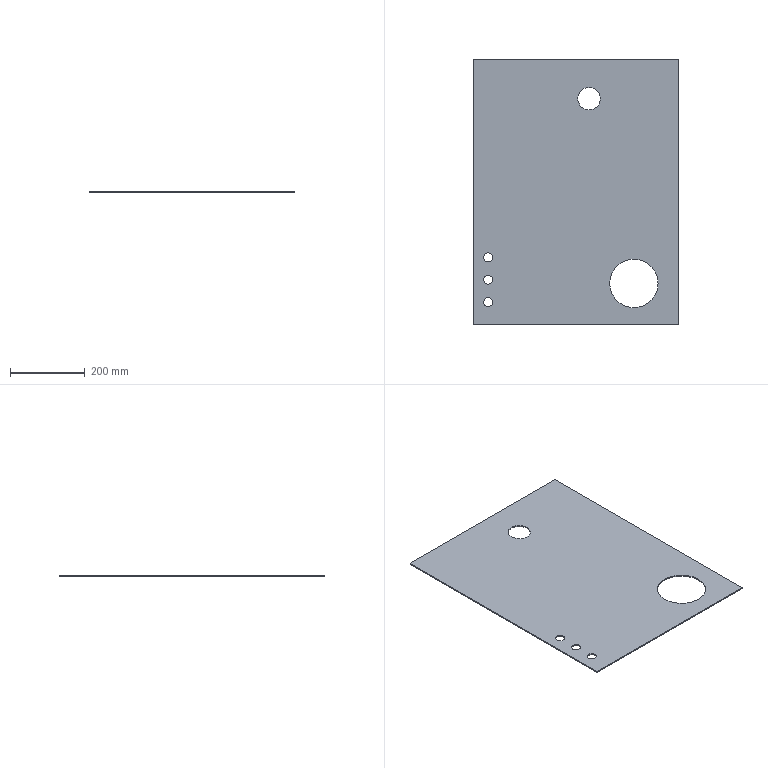Part | SolidWorks | features Extrusion 1 | 1 solid | 20 faces | box 550 x 710 x 3 mm | volume 1118991 mm3 | cylinder 14 | plane 6 | commonest cylinder face diameters 24.2 x6 4 x4 60.2 x2 130 x2
STEP:
#1=CARTESIAN_POINT('',(27.9,180.,3.));
#2=VERTEX_POINT('',#1);
#3=CARTESIAN_POINT('',(52.1,180.,3.));
#4=VERTEX_POINT('',#3);
#5=CARTESIAN_POINT('',(40.,180.,3.));
#6=DIRECTION('',(0.,0.,1.));
#7=DIRECTION('',(1.,0.,0.));
#8=AXIS2_PLACEMENT_3D('',#5,#6,#7);
#9=CIRCLE('',#8,12.1);
#10=EDGE_CURVE('',#2,#4,#9,.T.);
#11=ORIENTED_EDGE('',*,*,#10,.T.);
#12=CARTESIAN_POINT('',(52.1,180.,0.));
#13=VERTEX_POINT('',#12);
#14=CARTESIAN_POINT('',(52.1,180.,3.));
#15=DIRECTION('',(0.,0.,-1.));
#16=VECTOR('',#15,1000.);
#17=LINE('',#14,#16);
#18=EDGE_CURVE('',#4,#13,#17,.T.);
#19=ORIENTED_EDGE('',*,*,#18,.T.);
#20=CARTESIAN_POINT('',(27.9,180.,0.));
#21=VERTEX_POINT('',#20);
#22=CARTESIAN_POINT('',(40.,180.,0.));
#23=DIRECTION('',(0.,0.,1.));
#24=DIRECTION('',(1.,0.,0.));
#25=AXIS2_PLACEMENT_3D('',#22,#23,#24);
#26=CIRCLE('',#25,12.1);
#27=EDGE_CURVE('',#21,#13,#26,.T.);
#28=ORIENTED_EDGE('',*,*,#27,.F.);
#29=CARTESIAN_POINT('',(27.9,180.,3.));
#30=DIRECTION('',(0.,0.,-1.));
#31=VECTOR('',#30,1000.);
#32=LINE('',#29,#31);
#33=EDGE_CURVE('',#2,#21,#32,.T.);
#34=ORIENTED_EDGE('',*,*,#33,.F.);
#35=EDGE_LOOP('',(#11,#19,#28,#34));
#36=FACE_OUTER_BOUND('',#35,.T.);
#37=CARTESIAN_POINT('',(40.,180.,3.));
#38=DIRECTION('',(0.,0.,-1.));
#39=DIRECTION('',(-1.,0.,0.));
#40=AXIS2_PLACEMENT_3D('',#37,#38,#39);
#41=CYLINDRICAL_SURFACE('',#40,12.1);
#42=ADVANCED_FACE('',(#36),#41,.F.);
#43=CARTESIAN_POINT('',(27.9,120.,3.));
#44=VERTEX_POINT('',#43);
#45=CARTESIAN_POINT('',(52.1,120.,3.));
#46=VERTEX_POINT('',#45);
#47=CARTESIAN_POINT('',(40.,120.,3.));
#48=DIRECTION('',(0.,0.,1.));
#49=DIRECTION('',(1.,0.,0.));
#50=AXIS2_PLACEMENT_3D('',#47,#48,#49);
#51=CIRCLE('',#50,12.1);
#52=EDGE_CURVE('',#44,#46,#51,.T.);
#53=ORIENTED_EDGE('',*,*,#52,.T.);
#54=CARTESIAN_POINT('',(52.1,120.,0.));
#55=VERTEX_POINT('',#54);
#56=CARTESIAN_POINT('',(52.1,120.,3.));
#57=DIRECTION('',(0.,0.,-1.));
#58=VECTOR('',#57,1000.);
#59=LINE('',#56,#58);
#60=EDGE_CURVE('',#46,#55,#59,.T.);
#61=ORIENTED_EDGE('',*,*,#60,.T.);
#62=CARTESIAN_POINT('',(27.9,120.,0.));
#63=VERTEX_POINT('',#62);
#64=CARTESIAN_POINT('',(40.,120.,0.));
#65=DIRECTION('',(0.,0.,1.));
#66=DIRECTION('',(1.,0.,0.));
#67=AXIS2_PLACEMENT_3D('',#64,#65,#66);
#68=CIRCLE('',#67,12.1);
#69=EDGE_CURVE('',#63,#55,#68,.T.);
#70=ORIENTED_EDGE('',*,*,#69,.F.);
#71=CARTESIAN_POINT('',(27.9,120.,3.));
#72=DIRECTION('',(0.,0.,-1.));
#73=VECTOR('',#72,1000.);
#74=LINE('',#71,#73);
#75=EDGE_CURVE('',#44,#63,#74,.T.);
#76=ORIENTED_EDGE('',*,*,#75,.F.);
#77=EDGE_LOOP('',(#53,#61,#70,#76));
#78=FACE_OUTER_BOUND('',#77,.T.);
#79=CARTESIAN_POINT('',(40.,120.,3.));
#80=DIRECTION('',(0.,0.,-1.));
#81=DIRECTION('',(-1.,0.,0.));
#82=AXIS2_PLACEMENT_3D('',#79,#80,#81);
#83=CYLINDRICAL_SURFACE('',#82,12.1);
#84=ADVANCED_FACE('',(#78),#83,.F.);
#85=CARTESIAN_POINT('',(279.9,605.,3.));
#86=VERTEX_POINT('',#85);
#87=CARTESIAN_POINT('',(340.1,605.,3.));
#88=VERTEX_POINT('',#87);
#89=CARTESIAN_POINT('',(310.,605.,3.));
#90=DIRECTION('',(0.,0.,1.));
#91=DIRECTION('',(1.,0.,0.));
#92=AXIS2_PLACEMENT_3D('',#89,#90,#91);
#93=CIRCLE('',#92,30.1);
#94=EDGE_CURVE('',#86,#88,#93,.T.);
#95=ORIENTED_EDGE('',*,*,#94,.T.);
#96=CARTESIAN_POINT('',(340.1,605.,0.));
#97=VERTEX_POINT('',#96);
#98=CARTESIAN_POINT('',(340.1,605.,3.));
#99=DIRECTION('',(0.,0.,-1.));
#100=VECTOR('',#99,1000.);
#101=LINE('',#98,#100);
#102=EDGE_CURVE('',#88,#97,#101,.T.);
#103=ORIENTED_EDGE('',*,*,#102,.T.);
#104=CARTESIAN_POINT('',(279.9,605.,0.));
#105=VERTEX_POINT('',#104);
#106=CARTESIAN_POINT('',(310.,605.,0.));
#107=DIRECTION('',(0.,0.,1.));
#108=DIRECTION('',(1.,0.,0.));
#109=AXIS2_PLACEMENT_3D('',#106,#107,#108);
#110=CIRCLE('',#109,30.1);
#111=EDGE_CURVE('',#105,#97,#110,.T.);
#112=ORIENTED_EDGE('',*,*,#111,.F.);
#113=CARTESIAN_POINT('',(279.9,605.,3.));
#114=DIRECTION('',(0.,0.,-1.));
#115=VECTOR('',#114,1000.);
#116=LINE('',#113,#115);
#117=EDGE_CURVE('',#86,#105,#116,.T.);
#118=ORIENTED_EDGE('',*,*,#117,.F.);
#119=EDGE_LOOP('',(#95,#103,#112,#118));
#120=FACE_OUTER_BOUND('',#119,.T.);
#121=CARTESIAN_POINT('',(310.,605.,3.));
#122=DIRECTION('',(0.,0.,-1.));
#123=DIRECTION('',(-1.,0.,0.));
#124=AXIS2_PLACEMENT_3D('',#121,#122,#123);
#125=CYLINDRICAL_SURFACE('',#124,30.1);
#126=ADVANCED_FACE('',(#120),#125,.F.);
#127=CARTESIAN_POINT('',(365.,110.,3.));
#128=VERTEX_POINT('',#127);
#129=CARTESIAN_POINT('',(495.,110.,3.));
#130=VERTEX_POINT('',#129);
#131=CARTESIAN_POINT('',(430.,110.,3.));
#132=DIRECTION('',(0.,0.,1.));
#133=DIRECTION('',(1.,0.,0.));
#134=AXIS2_PLACEMENT_3D('',#131,#132,#133);
#135=CIRCLE('',#134,65.);
#136=EDGE_CURVE('',#128,#130,#135,.T.);
#137=ORIENTED_EDGE('',*,*,#136,.T.);
#138=CARTESIAN_POINT('',(495.,110.,0.));
#139=VERTEX_POINT('',#138);
#140=CARTESIAN_POINT('',(495.,110.,3.));
#141=DIRECTION('',(0.,0.,-1.));
#142=VECTOR('',#141,1000.);
#143=LINE('',#140,#142);
#144=EDGE_CURVE('',#130,#139,#143,.T.);
#145=ORIENTED_EDGE('',*,*,#144,.T.);
#146=CARTESIAN_POINT('',(365.,110.,0.));
#147=VERTEX_POINT('',#146);
#148=CARTESIAN_POINT('',(430.,110.,0.));
#149=DIRECTION('',(0.,0.,1.));
#150=DIRECTION('',(1.,0.,0.));
#151=AXIS2_PLACEMENT_3D('',#148,#149,#150);
#152=CIRCLE('',#151,65.);
#153=EDGE_CURVE('',#147,#139,#152,.T.);
#154=ORIENTED_EDGE('',*,*,#153,.F.);
#155=CARTESIAN_POINT('',(365.,110.,3.));
#156=DIRECTION('',(0.,0.,-1.));
#157=VECTOR('',#156,1000.);
#158=LINE('',#155,#157);
#159=EDGE_CURVE('',#128,#147,#158,.T.);
#160=ORIENTED_EDGE('',*,*,#159,.F.);
#161=EDGE_LOOP('',(#137,#145,#154,#160));
#162=FACE_OUTER_BOUND('',#161,.T.);
#163=CARTESIAN_POINT('',(430.,110.,3.));
#164=DIRECTION('',(0.,0.,-1.));
#165=DIRECTION('',(-1.,0.,0.));
#166=AXIS2_PLACEMENT_3D('',#163,#164,#165);
#167=CYLINDRICAL_SURFACE('',#166,65.);
#168=ADVANCED_FACE('',(#162),#167,.F.);
#169=CARTESIAN_POINT('',(27.9,60.,3.));
#170=VERTEX_POINT('',#169);
#171=CARTESIAN_POINT('',(52.1,60.,3.));
#172=VERTEX_POINT('',#171);
#173=CARTESIAN_POINT('',(40.,60.,3.));
#174=DIRECTION('',(0.,0.,1.));
#175=DIRECTION('',(1.,0.,0.));
#176=AXIS2_PLACEMENT_3D('',#173,#174,#175);
#177=CIRCLE('',#176,12.1);
#178=EDGE_CURVE('',#170,#172,#177,.T.);
#179=ORIENTED_EDGE('',*,*,#178,.T.);
#180=CARTESIAN_POINT('',(52.1,60.,0.));
#181=VERTEX_POINT('',#180);
#182=CARTESIAN_POINT('',(52.1,60.,3.));
#183=DIRECTION('',(0.,0.,-1.));
#184=VECTOR('',#183,1000.);
#185=LINE('',#182,#184);
#186=EDGE_CURVE('',#172,#181,#185,.T.);
#187=ORIENTED_EDGE('',*,*,#186,.T.);
#188=CARTESIAN_POINT('',(27.9,60.,0.));
#189=VERTEX_POINT('',#188);
#190=CARTESIAN_POINT('',(40.,60.,0.));
#191=DIRECTION('',(0.,0.,1.));
#192=DIRECTION('',(1.,0.,0.));
#193=AXIS2_PLACEMENT_3D('',#190,#191,#192);
#194=CIRCLE('',#193,12.1);
#195=EDGE_CURVE('',#189,#181,#194,.T.);
#196=ORIENTED_EDGE('',*,*,#195,.F.);
#197=CARTESIAN_POINT('',(27.9,60.,3.));
#198=DIRECTION('',(0.,0.,-1.));
#199=VECTOR('',#198,1000.);
#200=LINE('',#197,#199);
#201=EDGE_CURVE('',#170,#189,#200,.T.);
#202=ORIENTED_EDGE('',*,*,#201,.F.);
#203=EDGE_LOOP('',(#179,#187,#196,#202));
#204=FACE_OUTER_BOUND('',#203,.T.);
#205=CARTESIAN_POINT('',(40.,60.,3.));
#206=DIRECTION('',(0.,0.,-1.));
#207=DIRECTION('',(-1.,0.,0.));
#208=AXIS2_PLACEMENT_3D('',#205,#206,#207);
#209=CYLINDRICAL_SURFACE('',#208,12.1);
#210=ADVANCED_FACE('',(#204),#209,.F.);
#211=CARTESIAN_POINT('',(2.,710.,3.));
#212=VERTEX_POINT('',#211);
#213=CARTESIAN_POINT('',(0.,708.,3.));
#214=VERTEX_POINT('',#213);
#215=CARTESIAN_POINT('',(2.,708.,3.));
#216=DIRECTION('',(0.,0.,1.));
#217=DIRECTION('',(-1.,0.,0.));
#218=AXIS2_PLACEMENT_3D('',#215,#216,#217);
#219=CIRCLE('',#218,2.);
#220=EDGE_CURVE('',#212,#214,#219,.T.);
#221=ORIENTED_EDGE('',*,*,#220,.T.);
#222=CARTESIAN_POINT('',(0.,2.,3.));
#223=VERTEX_POINT('',#222);
#224=CARTESIAN_POINT('',(0.,2.,3.));
#225=DIRECTION('',(0.,-1.,0.));
#226=VECTOR('',#225,1000.);
#227=LINE('',#224,#226);
#228=EDGE_CURVE('',#214,#223,#227,.T.);
#229=ORIENTED_EDGE('',*,*,#228,.T.);
#230=CARTESIAN_POINT('',(2.,0.,3.));
#231=VERTEX_POINT('',#230);
#232=CARTESIAN_POINT('',(2.,2.,3.));
#233=DIRECTION('',(0.,0.,1.));
#234=DIRECTION('',(-1.,0.,0.));
#235=AXIS2_PLACEMENT_3D('',#232,#233,#234);
#236=CIRCLE('',#235,2.);
#237=EDGE_CURVE('',#223,#231,#236,.T.);
#238=ORIENTED_EDGE('',*,*,#237,.T.);
#239=CARTESIAN_POINT('',(548.,0.,3.));
#240=VERTEX_POINT('',#239);
#241=CARTESIAN_POINT('',(2.,0.,3.));
#242=DIRECTION('',(1.,0.,0.));
#243=VECTOR('',#242,1000.);
#244=LINE('',#241,#243);
#245=EDGE_CURVE('',#231,#240,#244,.T.);
#246=ORIENTED_EDGE('',*,*,#245,.T.);
#247=CARTESIAN_POINT('',(550.,2.,3.));
#248=VERTEX_POINT('',#247);
#249=CARTESIAN_POINT('',(548.,2.,3.));
#250=DIRECTION('',(0.,0.,1.));
#251=DIRECTION('',(1.,0.,0.));
#252=AXIS2_PLACEMENT_3D('',#249,#250,#251);
#253=CIRCLE('',#252,2.);
#254=EDGE_CURVE('',#240,#248,#253,.T.);
#255=ORIENTED_EDGE('',*,*,#254,.T.);
#256=CARTESIAN_POINT('',(550.,708.,3.));
#257=VERTEX_POINT('',#256);
#258=CARTESIAN_POINT('',(550.,2.,3.));
#259=DIRECTION('',(0.,1.,0.));
#260=VECTOR('',#259,1000.);
#261=LINE('',#258,#260);
#262=EDGE_CURVE('',#248,#257,#261,.T.);
#263=ORIENTED_EDGE('',*,*,#262,.T.);
#264=CARTESIAN_POINT('',(548.,710.,3.));
#265=VERTEX_POINT('',#264);
#266=CARTESIAN_POINT('',(548.,708.,3.));
#267=DIRECTION('',(0.,0.,1.));
#268=DIRECTION('',(-1.,0.,0.));
#269=AXIS2_PLACEMENT_3D('',#266,#267,#268);
#270=CIRCLE('',#269,2.);
#271=EDGE_CURVE('',#257,#265,#270,.T.);
#272=ORIENTED_EDGE('',*,*,#271,.T.);
#273=CARTESIAN_POINT('',(2.,710.,3.));
#274=DIRECTION('',(-1.,0.,0.));
#275=VECTOR('',#274,1000.);
#276=LINE('',#273,#275);
#277=EDGE_CURVE('',#265,#212,#276,.T.);
#278=ORIENTED_EDGE('',*,*,#277,.T.);
#279=EDGE_LOOP('',(#221,#229,#238,#246,#255,#263,#272,#278));
#280=FACE_OUTER_BOUND('',#279,.T.);
#281=ORIENTED_EDGE('',*,*,#178,.F.);
#282=CARTESIAN_POINT('',(40.,60.,3.));
#283=DIRECTION('',(0.,0.,1.));
#284=DIRECTION('',(1.,0.,0.));
#285=AXIS2_PLACEMENT_3D('',#282,#283,#284);
#286=CIRCLE('',#285,12.1);
#287=EDGE_CURVE('',#172,#170,#286,.T.);
#288=ORIENTED_EDGE('',*,*,#287,.F.);
#289=EDGE_LOOP('',(#281,#288));
#290=FACE_BOUND('',#289,.T.);
#291=ORIENTED_EDGE('',*,*,#136,.F.);
#292=CARTESIAN_POINT('',(430.,110.,3.));
#293=DIRECTION('',(0.,0.,1.));
#294=DIRECTION('',(1.,0.,0.));
#295=AXIS2_PLACEMENT_3D('',#292,#293,#294);
#296=CIRCLE('',#295,65.);
#297=EDGE_CURVE('',#130,#128,#296,.T.);
#298=ORIENTED_EDGE('',*,*,#297,.F.);
#299=EDGE_LOOP('',(#291,#298));
#300=FACE_BOUND('',#299,.T.);
#301=ORIENTED_EDGE('',*,*,#94,.F.);
#302=CARTESIAN_POINT('',(310.,605.,3.));
#303=DIRECTION('',(0.,0.,1.));
#304=DIRECTION('',(1.,0.,0.));
#305=AXIS2_PLACEMENT_3D('',#302,#303,#304);
#306=CIRCLE('',#305,30.1);
#307=EDGE_CURVE('',#88,#86,#306,.T.);
#308=ORIENTED_EDGE('',*,*,#307,.F.);
#309=EDGE_LOOP('',(#301,#308));
#310=FACE_BOUND('',#309,.T.);
#311=ORIENTED_EDGE('',*,*,#52,.F.);
#312=CARTESIAN_POINT('',(40.,120.,3.));
#313=DIRECTION('',(0.,0.,1.));
#314=DIRECTION('',(1.,0.,0.));
#315=AXIS2_PLACEMENT_3D('',#312,#313,#314);
#316=CIRCLE('',#315,12.1);
#317=EDGE_CURVE('',#46,#44,#316,.T.);
#318=ORIENTED_EDGE('',*,*,#317,.F.);
#319=EDGE_LOOP('',(#311,#318));
#320=FACE_BOUND('',#319,.T.);
#321=ORIENTED_EDGE('',*,*,#10,.F.);
#322=CARTESIAN_POINT('',(40.,180.,3.));
#323=DIRECTION('',(0.,0.,1.));
#324=DIRECTION('',(1.,0.,0.));
#325=AXIS2_PLACEMENT_3D('',#322,#323,#324);
#326=CIRCLE('',#325,12.1);
#327=EDGE_CURVE('',#4,#2,#326,.T.);
#328=ORIENTED_EDGE('',*,*,#327,.F.);
#329=EDGE_LOOP('',(#321,#328));
#330=FACE_BOUND('',#329,.T.);
#331=CARTESIAN_POINT('',(2.,708.,3.));
#332=DIRECTION('',(0.,0.,-1.));
#333=DIRECTION('',(-1.,0.,0.));
#334=AXIS2_PLACEMENT_3D('',#331,#332,#333);
#335=PLANE('',#334);
#336=ADVANCED_FACE('',(#280,#290,#300,#310,#320,#330),#335,.F.);
#337=ORIENTED_EDGE('',*,*,#69,.T.);
#338=CARTESIAN_POINT('',(40.,120.,0.));
#339=DIRECTION('',(0.,0.,1.));
#340=DIRECTION('',(1.,0.,0.));
#341=AXIS2_PLACEMENT_3D('',#338,#339,#340);
#342=CIRCLE('',#341,12.1);
#343=EDGE_CURVE('',#55,#63,#342,.T.);
#344=ORIENTED_EDGE('',*,*,#343,.T.);
#345=EDGE_LOOP('',(#337,#344));
#346=FACE_BOUND('',#345,.T.);
#347=ORIENTED_EDGE('',*,*,#153,.T.);
#348=CARTESIAN_POINT('',(430.,110.,0.));
#349=DIRECTION('',(0.,0.,1.));
#350=DIRECTION('',(1.,0.,0.));
#351=AXIS2_PLACEMENT_3D('',#348,#349,#350);
#352=CIRCLE('',#351,65.);
#353=EDGE_CURVE('',#139,#147,#352,.T.);
#354=ORIENTED_EDGE('',*,*,#353,.T.);
#355=EDGE_LOOP('',(#347,#354));
#356=FACE_BOUND('',#355,.T.);
#357=CARTESIAN_POINT('',(2.,710.,0.));
#358=VERTEX_POINT('',#357);
#359=CARTESIAN_POINT('',(0.,708.,0.));
#360=VERTEX_POINT('',#359);
#361=CARTESIAN_POINT('',(2.,708.,0.));
#362=DIRECTION('',(0.,0.,1.));
#363=DIRECTION('',(-1.,0.,0.));
#364=AXIS2_PLACEMENT_3D('',#361,#362,#363);
#365=CIRCLE('',#364,2.);
#366=EDGE_CURVE('',#358,#360,#365,.T.);
#367=ORIENTED_EDGE('',*,*,#366,.F.);
#368=CARTESIAN_POINT('',(548.,710.,0.));
#369=VERTEX_POINT('',#368);
#370=CARTESIAN_POINT('',(2.,710.,0.));
#371=DIRECTION('',(-1.,0.,0.));
#372=VECTOR('',#371,1000.);
#373=LINE('',#370,#372);
#374=EDGE_CURVE('',#369,#358,#373,.T.);
#375=ORIENTED_EDGE('',*,*,#374,.F.);
#376=CARTESIAN_POINT('',(550.,708.,0.));
#377=VERTEX_POINT('',#376);
#378=CARTESIAN_POINT('',(548.,708.,0.));
#379=DIRECTION('',(0.,0.,1.));
#380=DIRECTION('',(-1.,0.,0.));
#381=AXIS2_PLACEMENT_3D('',#378,#379,#380);
#382=CIRCLE('',#381,2.);
#383=EDGE_CURVE('',#377,#369,#382,.T.);
#384=ORIENTED_EDGE('',*,*,#383,.F.);
#385=CARTESIAN_POINT('',(550.,2.,0.));
#386=VERTEX_POINT('',#385);
#387=CARTESIAN_POINT('',(550.,2.,0.));
#388=DIRECTION('',(0.,1.,0.));
#389=VECTOR('',#388,1000.);
#390=LINE('',#387,#389);
#391=EDGE_CURVE('',#386,#377,#390,.T.);
#392=ORIENTED_EDGE('',*,*,#391,.F.);
#393=CARTESIAN_POINT('',(548.,0.,0.));
#394=VERTEX_POINT('',#393);
#395=CARTESIAN_POINT('',(548.,2.,0.));
#396=DIRECTION('',(0.,0.,1.));
#397=DIRECTION('',(1.,0.,0.));
#398=AXIS2_PLACEMENT_3D('',#395,#396,#397);
#399=CIRCLE('',#398,2.);
#400=EDGE_CURVE('',#394,#386,#399,.T.);
#401=ORIENTED_EDGE('',*,*,#400,.F.);
#402=CARTESIAN_POINT('',(2.,0.,0.));
#403=VERTEX_POINT('',#402);
#404=CARTESIAN_POINT('',(2.,0.,0.));
#405=DIRECTION('',(1.,0.,0.));
#406=VECTOR('',#405,1000.);
#407=LINE('',#404,#406);
#408=EDGE_CURVE('',#403,#394,#407,.T.);
#409=ORIENTED_EDGE('',*,*,#408,.F.);
#410=CARTESIAN_POINT('',(0.,2.,0.));
#411=VERTEX_POINT('',#410);
#412=CARTESIAN_POINT('',(2.,2.,0.));
#413=DIRECTION('',(0.,0.,1.));
#414=DIRECTION('',(-1.,0.,0.));
#415=AXIS2_PLACEMENT_3D('',#412,#413,#414);
#416=CIRCLE('',#415,2.);
#417=EDGE_CURVE('',#411,#403,#416,.T.);
#418=ORIENTED_EDGE('',*,*,#417,.F.);
#419=CARTESIAN_POINT('',(0.,2.,0.));
#420=DIRECTION('',(0.,-1.,0.));
#421=VECTOR('',#420,1000.);
#422=LINE('',#419,#421);
#423=EDGE_CURVE('',#360,#411,#422,.T.);
#424=ORIENTED_EDGE('',*,*,#423,.F.);
#425=EDGE_LOOP('',(#367,#375,#384,#392,#401,#409,#418,#424));
#426=FACE_OUTER_BOUND('',#425,.T.);
#427=ORIENTED_EDGE('',*,*,#195,.T.);
#428=CARTESIAN_POINT('',(40.,60.,0.));
#429=DIRECTION('',(0.,0.,1.));
#430=DIRECTION('',(1.,0.,0.));
#431=AXIS2_PLACEMENT_3D('',#428,#429,#430);
#432=CIRCLE('',#431,12.1);
#433=EDGE_CURVE('',#181,#189,#432,.T.);
#434=ORIENTED_EDGE('',*,*,#433,.T.);
#435=EDGE_LOOP('',(#427,#434));
#436=FACE_BOUND('',#435,.T.);
#437=ORIENTED_EDGE('',*,*,#111,.T.);
#438=CARTESIAN_POINT('',(310.,605.,0.));
#439=DIRECTION('',(0.,0.,1.));
#440=DIRECTION('',(1.,0.,0.));
#441=AXIS2_PLACEMENT_3D('',#438,#439,#440);
#442=CIRCLE('',#441,30.1);
#443=EDGE_CURVE('',#97,#105,#442,.T.);
#444=ORIENTED_EDGE('',*,*,#443,.T.);
#445=EDGE_LOOP('',(#437,#444));
#446=FACE_BOUND('',#445,.T.);
#447=ORIENTED_EDGE('',*,*,#27,.T.);
#448=CARTESIAN_POINT('',(40.,180.,0.));
#449=DIRECTION('',(0.,0.,1.));
#450=DIRECTION('',(1.,0.,0.));
#451=AXIS2_PLACEMENT_3D('',#448,#449,#450);
#452=CIRCLE('',#451,12.1);
#453=EDGE_CURVE('',#13,#21,#452,.T.);
#454=ORIENTED_EDGE('',*,*,#453,.T.);
#455=EDGE_LOOP('',(#447,#454));
#456=FACE_BOUND('',#455,.T.);
#457=CARTESIAN_POINT('',(2.,708.,0.));
#458=DIRECTION('',(0.,0.,-1.));
#459=DIRECTION('',(-1.,0.,0.));
#460=AXIS2_PLACEMENT_3D('',#457,#458,#459);
#461=PLANE('',#460);
#462=ADVANCED_FACE('',(#346,#356,#426,#436,#446,#456),#461,.T.);
#463=ORIENTED_EDGE('',*,*,#366,.T.);
#464=CARTESIAN_POINT('',(0.,708.,3.));
#465=DIRECTION('',(0.,0.,-1.));
#466=VECTOR('',#465,1000.);
#467=LINE('',#464,#466);
#468=EDGE_CURVE('',#214,#360,#467,.T.);
#469=ORIENTED_EDGE('',*,*,#468,.F.);
#470=ORIENTED_EDGE('',*,*,#220,.F.);
#471=CARTESIAN_POINT('',(2.,710.,3.));
#472=DIRECTION('',(0.,0.,-1.));
#473=VECTOR('',#472,1000.);
#474=LINE('',#471,#473);
#475=EDGE_CURVE('',#212,#358,#474,.T.);
#476=ORIENTED_EDGE('',*,*,#475,.T.);
#477=EDGE_LOOP('',(#463,#469,#470,#476));
#478=FACE_OUTER_BOUND('',#477,.T.);
#479=CARTESIAN_POINT('',(2.,708.,3.));
#480=DIRECTION('',(0.,0.,-1.));
#481=DIRECTION('',(-1.,0.,0.));
#482=AXIS2_PLACEMENT_3D('',#479,#480,#481);
#483=CYLINDRICAL_SURFACE('',#482,2.);
#484=ADVANCED_FACE('',(#478),#483,.T.);
#485=ORIENTED_EDGE('',*,*,#423,.T.);
#486=CARTESIAN_POINT('',(0.,2.,3.));
#487=DIRECTION('',(0.,0.,-1.));
#488=VECTOR('',#487,1000.);
#489=LINE('',#486,#488);
#490=EDGE_CURVE('',#223,#411,#489,.T.);
#491=ORIENTED_EDGE('',*,*,#490,.F.);
#492=ORIENTED_EDGE('',*,*,#228,.F.);
#493=ORIENTED_EDGE('',*,*,#468,.T.);
#494=EDGE_LOOP('',(#485,#491,#492,#493));
#495=FACE_OUTER_BOUND('',#494,.T.);
#496=CARTESIAN_POINT('',(0.,2.,3.));
#497=DIRECTION('',(1.,0.,0.));
#498=DIRECTION('',(0.,0.,-1.));
#499=AXIS2_PLACEMENT_3D('',#496,#497,#498);
#500=PLANE('',#499);
#501=ADVANCED_FACE('',(#495),#500,.F.);
#502=ORIENTED_EDGE('',*,*,#417,.T.);
#503=CARTESIAN_POINT('',(2.,0.,3.));
#504=DIRECTION('',(0.,0.,-1.));
#505=VECTOR('',#504,1000.);
#506=LINE('',#503,#505);
#507=EDGE_CURVE('',#231,#403,#506,.T.);
#508=ORIENTED_EDGE('',*,*,#507,.F.);
#509=ORIENTED_EDGE('',*,*,#237,.F.);
#510=ORIENTED_EDGE('',*,*,#490,.T.);
#511=EDGE_LOOP('',(#502,#508,#509,#510));
#512=FACE_OUTER_BOUND('',#511,.T.);
#513=CARTESIAN_POINT('',(2.,2.,3.));
#514=DIRECTION('',(0.,0.,-1.));
#515=DIRECTION('',(-1.,0.,0.));
#516=AXIS2_PLACEMENT_3D('',#513,#514,#515);
#517=CYLINDRICAL_SURFACE('',#516,2.);
#518=ADVANCED_FACE('',(#512),#517,.T.);
#519=ORIENTED_EDGE('',*,*,#408,.T.);
#520=CARTESIAN_POINT('',(548.,0.,3.));
#521=DIRECTION('',(0.,0.,-1.));
#522=VECTOR('',#521,1000.);
#523=LINE('',#520,#522);
#524=EDGE_CURVE('',#240,#394,#523,.T.);
#525=ORIENTED_EDGE('',*,*,#524,.F.);
#526=ORIENTED_EDGE('',*,*,#245,.F.);
#527=ORIENTED_EDGE('',*,*,#507,.T.);
#528=EDGE_LOOP('',(#519,#525,#526,#527));
#529=FACE_OUTER_BOUND('',#528,.T.);
#530=CARTESIAN_POINT('',(2.,0.,3.));
#531=DIRECTION('',(0.,1.,0.));
#532=DIRECTION('',(0.,0.,1.));
#533=AXIS2_PLACEMENT_3D('',#530,#531,#532);
#534=PLANE('',#533);
#535=ADVANCED_FACE('',(#529),#534,.F.);
#536=ORIENTED_EDGE('',*,*,#400,.T.);
#537=CARTESIAN_POINT('',(550.,2.,3.));
#538=DIRECTION('',(0.,0.,-1.));
#539=VECTOR('',#538,1000.);
#540=LINE('',#537,#539);
#541=EDGE_CURVE('',#248,#386,#540,.T.);
#542=ORIENTED_EDGE('',*,*,#541,.F.);
#543=ORIENTED_EDGE('',*,*,#254,.F.);
#544=ORIENTED_EDGE('',*,*,#524,.T.);
#545=EDGE_LOOP('',(#536,#542,#543,#544));
#546=FACE_OUTER_BOUND('',#545,.T.);
#547=CARTESIAN_POINT('',(548.,2.,3.));
#548=DIRECTION('',(0.,0.,-1.));
#549=DIRECTION('',(-1.,0.,0.));
#550=AXIS2_PLACEMENT_3D('',#547,#548,#549);
#551=CYLINDRICAL_SURFACE('',#550,2.);
#552=ADVANCED_FACE('',(#546),#551,.T.);
#553=ORIENTED_EDGE('',*,*,#391,.T.);
#554=CARTESIAN_POINT('',(550.,708.,3.));
#555=DIRECTION('',(0.,0.,-1.));
#556=VECTOR('',#555,1000.);
#557=LINE('',#554,#556);
#558=EDGE_CURVE('',#257,#377,#557,.T.);
#559=ORIENTED_EDGE('',*,*,#558,.F.);
#560=ORIENTED_EDGE('',*,*,#262,.F.);
#561=ORIENTED_EDGE('',*,*,#541,.T.);
#562=EDGE_LOOP('',(#553,#559,#560,#561));
#563=FACE_OUTER_BOUND('',#562,.T.);
#564=CARTESIAN_POINT('',(550.,2.,3.));
#565=DIRECTION('',(-1.,0.,0.));
#566=DIRECTION('',(0.,0.,1.));
#567=AXIS2_PLACEMENT_3D('',#564,#565,#566);
#568=PLANE('',#567);
#569=ADVANCED_FACE('',(#563),#568,.F.);
#570=ORIENTED_EDGE('',*,*,#383,.T.);
#571=CARTESIAN_POINT('',(548.,710.,3.));
#572=DIRECTION('',(0.,0.,-1.));
#573=VECTOR('',#572,1000.);
#574=LINE('',#571,#573);
#575=EDGE_CURVE('',#265,#369,#574,.T.);
#576=ORIENTED_EDGE('',*,*,#575,.F.);
#577=ORIENTED_EDGE('',*,*,#271,.F.);
#578=ORIENTED_EDGE('',*,*,#558,.T.);
#579=EDGE_LOOP('',(#570,#576,#577,#578));
#580=FACE_OUTER_BOUND('',#579,.T.);
#581=CARTESIAN_POINT('',(548.,708.,3.));
#582=DIRECTION('',(0.,0.,-1.));
#583=DIRECTION('',(-1.,0.,0.));
#584=AXIS2_PLACEMENT_3D('',#581,#582,#583);
#585=CYLINDRICAL_SURFACE('',#584,2.);
#586=ADVANCED_FACE('',(#580),#585,.T.);
#587=ORIENTED_EDGE('',*,*,#374,.T.);
#588=ORIENTED_EDGE('',*,*,#475,.F.);
#589=ORIENTED_EDGE('',*,*,#277,.F.);
#590=ORIENTED_EDGE('',*,*,#575,.T.);
#591=EDGE_LOOP('',(#587,#588,#589,#590));
#592=FACE_OUTER_BOUND('',#591,.T.);
#593=CARTESIAN_POINT('',(2.,710.,3.));
#594=DIRECTION('',(0.,-1.,0.));
#595=DIRECTION('',(0.,0.,-1.));
#596=AXIS2_PLACEMENT_3D('',#593,#594,#595);
#597=PLANE('',#596);
#598=ADVANCED_FACE('',(#592),#597,.F.);
#599=ORIENTED_EDGE('',*,*,#186,.F.);
#600=ORIENTED_EDGE('',*,*,#287,.T.);
#601=ORIENTED_EDGE('',*,*,#201,.T.);
#602=ORIENTED_EDGE('',*,*,#433,.F.);
#603=EDGE_LOOP('',(#599,#600,#601,#602));
#604=FACE_OUTER_BOUND('',#603,.T.);
#605=CARTESIAN_POINT('',(40.,60.,3.));
#606=DIRECTION('',(0.,0.,-1.));
#607=DIRECTION('',(-1.,0.,0.));
#608=AXIS2_PLACEMENT_3D('',#605,#606,#607);
#609=CYLINDRICAL_SURFACE('',#608,12.1);
#610=ADVANCED_FACE('',(#604),#609,.F.);
#611=ORIENTED_EDGE('',*,*,#144,.F.);
#612=ORIENTED_EDGE('',*,*,#297,.T.);
#613=ORIENTED_EDGE('',*,*,#159,.T.);
#614=ORIENTED_EDGE('',*,*,#353,.F.);
#615=EDGE_LOOP('',(#611,#612,#613,#614));
#616=FACE_OUTER_BOUND('',#615,.T.);
#617=CARTESIAN_POINT('',(430.,110.,3.));
#618=DIRECTION('',(0.,0.,-1.));
#619=DIRECTION('',(-1.,0.,0.));
#620=AXIS2_PLACEMENT_3D('',#617,#618,#619);
#621=CYLINDRICAL_SURFACE('',#620,65.);
#622=ADVANCED_FACE('',(#616),#621,.F.);
#623=ORIENTED_EDGE('',*,*,#102,.F.);
#624=ORIENTED_EDGE('',*,*,#307,.T.);
#625=ORIENTED_EDGE('',*,*,#117,.T.);
#626=ORIENTED_EDGE('',*,*,#443,.F.);
#627=EDGE_LOOP('',(#623,#624,#625,#626));
#628=FACE_OUTER_BOUND('',#627,.T.);
#629=CARTESIAN_POINT('',(310.,605.,3.));
#630=DIRECTION('',(0.,0.,-1.));
#631=DIRECTION('',(-1.,0.,0.));
#632=AXIS2_PLACEMENT_3D('',#629,#630,#631);
#633=CYLINDRICAL_SURFACE('',#632,30.1);
#634=ADVANCED_FACE('',(#628),#633,.F.);
#635=ORIENTED_EDGE('',*,*,#60,.F.);
#636=ORIENTED_EDGE('',*,*,#317,.T.);
#637=ORIENTED_EDGE('',*,*,#75,.T.);
#638=ORIENTED_EDGE('',*,*,#343,.F.);
#639=EDGE_LOOP('',(#635,#636,#637,#638));
#640=FACE_OUTER_BOUND('',#639,.T.);
#641=CARTESIAN_POINT('',(40.,120.,3.));
#642=DIRECTION('',(0.,0.,-1.));
#643=DIRECTION('',(-1.,0.,0.));
#644=AXIS2_PLACEMENT_3D('',#641,#642,#643);
#645=CYLINDRICAL_SURFACE('',#644,12.1);
#646=ADVANCED_FACE('',(#640),#645,.F.);
#647=ORIENTED_EDGE('',*,*,#18,.F.);
#648=ORIENTED_EDGE('',*,*,#327,.T.);
#649=ORIENTED_EDGE('',*,*,#33,.T.);
#650=ORIENTED_EDGE('',*,*,#453,.F.);
#651=EDGE_LOOP('',(#647,#648,#649,#650));
#652=FACE_OUTER_BOUND('',#651,.T.);
#653=CARTESIAN_POINT('',(40.,180.,3.));
#654=DIRECTION('',(0.,0.,-1.));
#655=DIRECTION('',(-1.,0.,0.));
#656=AXIS2_PLACEMENT_3D('',#653,#654,#655);
#657=CYLINDRICAL_SURFACE('',#656,12.1);
#658=ADVANCED_FACE('',(#652),#657,.F.);
#659=CLOSED_SHELL('',(#42,#84,#126,#168,#210,#336,#462,#484,#501,#518,#535,#552,#569,#586,#598,#610,#622,#634,#646,#658));
#660=MANIFOLD_SOLID_BREP('',#659);
#661=CARTESIAN_POINT('',(0.,0.,0.));
#662=DIRECTION('',(0.,0.,1.));
#663=DIRECTION('',(1.,0.,0.));
#664=AXIS2_PLACEMENT_3D('',#661,#662,#663);
#665=(LENGTH_UNIT()NAMED_UNIT(*)SI_UNIT(.MILLI.,.METRE.));
#666=UNCERTAINTY_MEASURE_WITH_UNIT(LENGTH_MEASURE(0.00001),#665,'','');
#667=(NAMED_UNIT(*)PLANE_ANGLE_UNIT()SI_UNIT($,.RADIAN.));
#668=(NAMED_UNIT(*)SI_UNIT($,.STERADIAN.)SOLID_ANGLE_UNIT());
#669=(GEOMETRIC_REPRESENTATION_CONTEXT(3)GLOBAL_UNCERTAINTY_ASSIGNED_CONTEXT((#666))GLOBAL_UNIT_ASSIGNED_CONTEXT((#665,#667,#668))REPRESENTATION_CONTEXT('',''));
#670=ADVANCED_BREP_SHAPE_REPRESENTATION('',(#660,#664),#669);